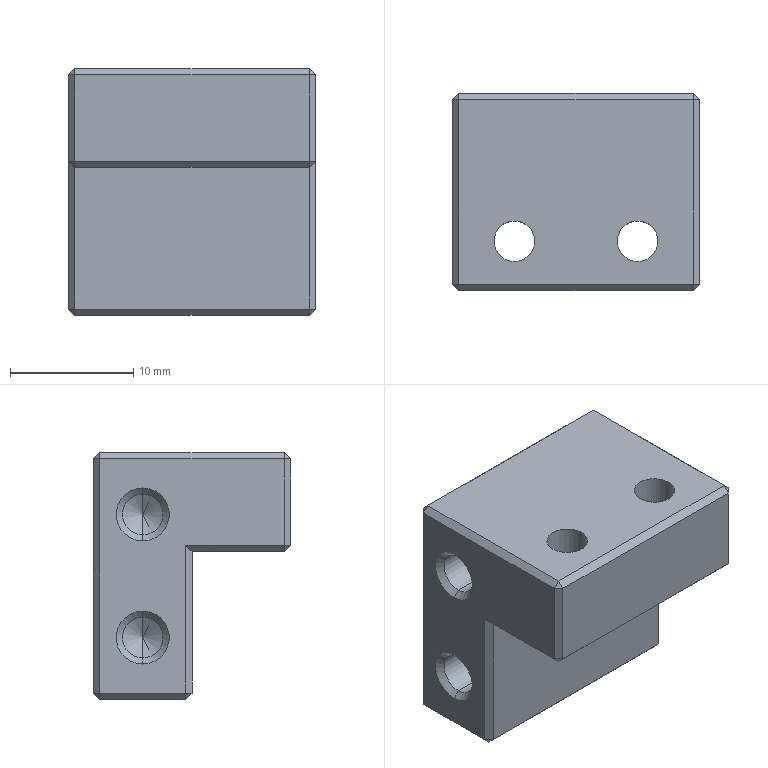Part | SolidWorks | features HoleWzd 2, Chamfer 1, Extrusion 1, ICE 1 | 1 solid | 51 faces | box 20 x 16 x 20 mm | volume 4064 mm3 | plane 35 | cone 8 | cylinder 8 | commonest cylinder face diameters 3.3 x8
STEP:
#1=CARTESIAN_POINT('',(-9.5,4.,-6.65));
#2=VERTEX_POINT('',#1);
#3=CARTESIAN_POINT('',(-9.5,4.,-3.35));
#4=VERTEX_POINT('',#3);
#5=CARTESIAN_POINT('',(-9.5,4.,-5.));
#6=DIRECTION('',(-1.,0.,0.));
#7=DIRECTION('',(0.,0.,-1.));
#8=AXIS2_PLACEMENT_3D('',#5,#6,#7);
#9=CIRCLE('',#8,1.65);
#10=EDGE_CURVE('',#2,#4,#9,.T.);
#11=ORIENTED_EDGE('',*,*,#10,.F.);
#12=CARTESIAN_POINT('',(-10.,4.,-7.15));
#13=VERTEX_POINT('',#12);
#14=CARTESIAN_POINT('',(-9.5,4.,-6.65));
#15=DIRECTION('',(-0.7071,0.,-0.7071));
#16=VECTOR('',#15,1000.);
#17=LINE('',#14,#16);
#18=EDGE_CURVE('',#2,#13,#17,.T.);
#19=ORIENTED_EDGE('',*,*,#18,.T.);
#20=CARTESIAN_POINT('',(-10.,4.,-2.85));
#21=VERTEX_POINT('',#20);
#22=CARTESIAN_POINT('',(-10.,4.,-5.));
#23=DIRECTION('',(1.,0.,0.));
#24=DIRECTION('',(0.,0.,-1.));
#25=AXIS2_PLACEMENT_3D('',#22,#23,#24);
#26=CIRCLE('',#25,2.15);
#27=EDGE_CURVE('',#21,#13,#26,.T.);
#28=ORIENTED_EDGE('',*,*,#27,.F.);
#29=CARTESIAN_POINT('',(-9.5,4.,-3.35));
#30=DIRECTION('',(-0.7071,0.,0.7071));
#31=VECTOR('',#30,1000.);
#32=LINE('',#29,#31);
#33=EDGE_CURVE('',#4,#21,#32,.T.);
#34=ORIENTED_EDGE('',*,*,#33,.F.);
#35=EDGE_LOOP('',(#11,#19,#28,#34));
#36=FACE_OUTER_BOUND('',#35,.T.);
#37=CARTESIAN_POINT('',(-9.5,4.,-5.));
#38=DIRECTION('',(-1.,0.,0.));
#39=DIRECTION('',(0.,0.,1.));
#40=AXIS2_PLACEMENT_3D('',#37,#38,#39);
#41=CONICAL_SURFACE('',#40,1.65,0.7854);
#42=ADVANCED_FACE('',(#36),#41,.F.);
#43=CARTESIAN_POINT('',(-9.5,4.,3.35));
#44=VERTEX_POINT('',#43);
#45=CARTESIAN_POINT('',(-9.5,4.,6.65));
#46=VERTEX_POINT('',#45);
#47=CARTESIAN_POINT('',(-9.5,4.,5.));
#48=DIRECTION('',(-1.,0.,0.));
#49=DIRECTION('',(0.,0.,-1.));
#50=AXIS2_PLACEMENT_3D('',#47,#48,#49);
#51=CIRCLE('',#50,1.65);
#52=EDGE_CURVE('',#44,#46,#51,.T.);
#53=ORIENTED_EDGE('',*,*,#52,.F.);
#54=CARTESIAN_POINT('',(-10.,4.,2.85));
#55=VERTEX_POINT('',#54);
#56=CARTESIAN_POINT('',(-9.5,4.,3.35));
#57=DIRECTION('',(-0.7071,0.,-0.7071));
#58=VECTOR('',#57,1000.);
#59=LINE('',#56,#58);
#60=EDGE_CURVE('',#44,#55,#59,.T.);
#61=ORIENTED_EDGE('',*,*,#60,.T.);
#62=CARTESIAN_POINT('',(-10.,4.,7.15));
#63=VERTEX_POINT('',#62);
#64=CARTESIAN_POINT('',(-10.,4.,5.));
#65=DIRECTION('',(1.,0.,0.));
#66=DIRECTION('',(0.,0.,-1.));
#67=AXIS2_PLACEMENT_3D('',#64,#65,#66);
#68=CIRCLE('',#67,2.15);
#69=EDGE_CURVE('',#63,#55,#68,.T.);
#70=ORIENTED_EDGE('',*,*,#69,.F.);
#71=CARTESIAN_POINT('',(-9.5,4.,6.65));
#72=DIRECTION('',(-0.7071,0.,0.7071));
#73=VECTOR('',#72,1000.);
#74=LINE('',#71,#73);
#75=EDGE_CURVE('',#46,#63,#74,.T.);
#76=ORIENTED_EDGE('',*,*,#75,.F.);
#77=EDGE_LOOP('',(#53,#61,#70,#76));
#78=FACE_OUTER_BOUND('',#77,.T.);
#79=CARTESIAN_POINT('',(-9.5,4.,5.));
#80=DIRECTION('',(-1.,0.,0.));
#81=DIRECTION('',(0.,0.,1.));
#82=AXIS2_PLACEMENT_3D('',#79,#80,#81);
#83=CONICAL_SURFACE('',#82,1.65,0.7854);
#84=ADVANCED_FACE('',(#78),#83,.F.);
#85=CARTESIAN_POINT('',(-6.65,-4.,2.));
#86=VERTEX_POINT('',#85);
#87=CARTESIAN_POINT('',(-3.35,-4.,2.));
#88=VERTEX_POINT('',#87);
#89=CARTESIAN_POINT('',(-5.,-4.,2.));
#90=DIRECTION('',(0.,0.,1.));
#91=DIRECTION('',(1.,0.,0.));
#92=AXIS2_PLACEMENT_3D('',#89,#90,#91);
#93=CIRCLE('',#92,1.65);
#94=EDGE_CURVE('',#86,#88,#93,.T.);
#95=ORIENTED_EDGE('',*,*,#94,.F.);
#96=CARTESIAN_POINT('',(-6.65,-4.,10.));
#97=VERTEX_POINT('',#96);
#98=CARTESIAN_POINT('',(-6.65,-4.,10.));
#99=DIRECTION('',(0.,0.,1.));
#100=VECTOR('',#99,1000.);
#101=LINE('',#98,#100);
#102=EDGE_CURVE('',#86,#97,#101,.T.);
#103=ORIENTED_EDGE('',*,*,#102,.T.);
#104=CARTESIAN_POINT('',(-3.35,-4.,10.));
#105=VERTEX_POINT('',#104);
#106=CARTESIAN_POINT('',(-5.,-4.,10.));
#107=DIRECTION('',(0.,0.,1.));
#108=DIRECTION('',(1.,0.,0.));
#109=AXIS2_PLACEMENT_3D('',#106,#107,#108);
#110=CIRCLE('',#109,1.65);
#111=EDGE_CURVE('',#97,#105,#110,.T.);
#112=ORIENTED_EDGE('',*,*,#111,.T.);
#113=CARTESIAN_POINT('',(-3.35,-4.,10.));
#114=DIRECTION('',(0.,0.,1.));
#115=VECTOR('',#114,1000.);
#116=LINE('',#113,#115);
#117=EDGE_CURVE('',#88,#105,#116,.T.);
#118=ORIENTED_EDGE('',*,*,#117,.F.);
#119=EDGE_LOOP('',(#95,#103,#112,#118));
#120=FACE_OUTER_BOUND('',#119,.T.);
#121=CARTESIAN_POINT('',(-5.,-4.,10.));
#122=DIRECTION('',(0.,0.,1.));
#123=DIRECTION('',(1.,0.,0.));
#124=AXIS2_PLACEMENT_3D('',#121,#122,#123);
#125=CYLINDRICAL_SURFACE('',#124,1.65);
#126=ADVANCED_FACE('',(#120),#125,.F.);
#127=CARTESIAN_POINT('',(3.35,-4.,2.));
#128=VERTEX_POINT('',#127);
#129=CARTESIAN_POINT('',(6.65,-4.,2.));
#130=VERTEX_POINT('',#129);
#131=CARTESIAN_POINT('',(5.,-4.,2.));
#132=DIRECTION('',(0.,0.,1.));
#133=DIRECTION('',(1.,0.,0.));
#134=AXIS2_PLACEMENT_3D('',#131,#132,#133);
#135=CIRCLE('',#134,1.65);
#136=EDGE_CURVE('',#128,#130,#135,.T.);
#137=ORIENTED_EDGE('',*,*,#136,.F.);
#138=CARTESIAN_POINT('',(3.35,-4.,10.));
#139=VERTEX_POINT('',#138);
#140=CARTESIAN_POINT('',(3.35,-4.,10.));
#141=DIRECTION('',(0.,0.,1.));
#142=VECTOR('',#141,1000.);
#143=LINE('',#140,#142);
#144=EDGE_CURVE('',#128,#139,#143,.T.);
#145=ORIENTED_EDGE('',*,*,#144,.T.);
#146=CARTESIAN_POINT('',(6.65,-4.,10.));
#147=VERTEX_POINT('',#146);
#148=CARTESIAN_POINT('',(5.,-4.,10.));
#149=DIRECTION('',(0.,0.,1.));
#150=DIRECTION('',(1.,0.,0.));
#151=AXIS2_PLACEMENT_3D('',#148,#149,#150);
#152=CIRCLE('',#151,1.65);
#153=EDGE_CURVE('',#139,#147,#152,.T.);
#154=ORIENTED_EDGE('',*,*,#153,.T.);
#155=CARTESIAN_POINT('',(6.65,-4.,10.));
#156=DIRECTION('',(0.,0.,1.));
#157=VECTOR('',#156,1000.);
#158=LINE('',#155,#157);
#159=EDGE_CURVE('',#130,#147,#158,.T.);
#160=ORIENTED_EDGE('',*,*,#159,.F.);
#161=EDGE_LOOP('',(#137,#145,#154,#160));
#162=FACE_OUTER_BOUND('',#161,.T.);
#163=CARTESIAN_POINT('',(5.,-4.,10.));
#164=DIRECTION('',(0.,0.,1.));
#165=DIRECTION('',(1.,0.,0.));
#166=AXIS2_PLACEMENT_3D('',#163,#164,#165);
#167=CYLINDRICAL_SURFACE('',#166,1.65);
#168=ADVANCED_FACE('',(#162),#167,.F.);
#169=CARTESIAN_POINT('',(4.1,4.,-6.65));
#170=VERTEX_POINT('',#169);
#171=CARTESIAN_POINT('',(4.1,4.,-3.35));
#172=VERTEX_POINT('',#171);
#173=CARTESIAN_POINT('',(4.1,4.,-5.));
#174=DIRECTION('',(-1.,0.,0.));
#175=DIRECTION('',(0.,0.,1.));
#176=AXIS2_PLACEMENT_3D('',#173,#174,#175);
#177=CIRCLE('',#176,1.65);
#178=EDGE_CURVE('',#170,#172,#177,.T.);
#179=ORIENTED_EDGE('',*,*,#178,.F.);
#180=CARTESIAN_POINT('',(-10.,4.,-6.65));
#181=DIRECTION('',(-1.,0.,0.));
#182=VECTOR('',#181,1000.);
#183=LINE('',#180,#182);
#184=EDGE_CURVE('',#170,#2,#183,.T.);
#185=ORIENTED_EDGE('',*,*,#184,.T.);
#186=ORIENTED_EDGE('',*,*,#10,.T.);
#187=CARTESIAN_POINT('',(-10.,4.,-3.35));
#188=DIRECTION('',(-1.,0.,0.));
#189=VECTOR('',#188,1000.);
#190=LINE('',#187,#189);
#191=EDGE_CURVE('',#172,#4,#190,.T.);
#192=ORIENTED_EDGE('',*,*,#191,.F.);
#193=EDGE_LOOP('',(#179,#185,#186,#192));
#194=FACE_OUTER_BOUND('',#193,.T.);
#195=CARTESIAN_POINT('',(-10.,4.,-5.));
#196=DIRECTION('',(-1.,0.,0.));
#197=DIRECTION('',(0.,0.,1.));
#198=AXIS2_PLACEMENT_3D('',#195,#196,#197);
#199=CYLINDRICAL_SURFACE('',#198,1.65);
#200=ADVANCED_FACE('',(#194),#199,.F.);
#201=CARTESIAN_POINT('',(5.091,4.,-5.));
#202=VERTEX_POINT('',#201);
#203=CARTESIAN_POINT('',(4.1,4.,-3.35));
#204=DIRECTION('',(-0.515,0.,0.8572));
#205=VECTOR('',#204,1000.);
#206=LINE('',#203,#205);
#207=EDGE_CURVE('',#202,#172,#206,.T.);
#208=ORIENTED_EDGE('',*,*,#207,.F.);
#209=CARTESIAN_POINT('',(4.1,4.,-6.65));
#210=DIRECTION('',(-0.515,0.,-0.8572));
#211=VECTOR('',#210,1000.);
#212=LINE('',#209,#211);
#213=EDGE_CURVE('',#202,#170,#212,.T.);
#214=ORIENTED_EDGE('',*,*,#213,.T.);
#215=ORIENTED_EDGE('',*,*,#178,.T.);
#216=EDGE_LOOP('',(#208,#214,#215));
#217=FACE_OUTER_BOUND('',#216,.T.);
#218=CARTESIAN_POINT('',(4.1,4.,-5.));
#219=DIRECTION('',(-1.,0.,0.));
#220=DIRECTION('',(0.,0.,1.));
#221=AXIS2_PLACEMENT_3D('',#218,#219,#220);
#222=CONICAL_SURFACE('',#221,1.65,1.03);
#223=ADVANCED_FACE('',(#217),#222,.F.);
#224=CARTESIAN_POINT('',(4.1,4.,3.35));
#225=VERTEX_POINT('',#224);
#226=CARTESIAN_POINT('',(4.1,4.,6.65));
#227=VERTEX_POINT('',#226);
#228=CARTESIAN_POINT('',(4.1,4.,5.));
#229=DIRECTION('',(-1.,0.,0.));
#230=DIRECTION('',(0.,0.,1.));
#231=AXIS2_PLACEMENT_3D('',#228,#229,#230);
#232=CIRCLE('',#231,1.65);
#233=EDGE_CURVE('',#225,#227,#232,.T.);
#234=ORIENTED_EDGE('',*,*,#233,.F.);
#235=CARTESIAN_POINT('',(-10.,4.,3.35));
#236=DIRECTION('',(-1.,0.,0.));
#237=VECTOR('',#236,1000.);
#238=LINE('',#235,#237);
#239=EDGE_CURVE('',#225,#44,#238,.T.);
#240=ORIENTED_EDGE('',*,*,#239,.T.);
#241=ORIENTED_EDGE('',*,*,#52,.T.);
#242=CARTESIAN_POINT('',(-10.,4.,6.65));
#243=DIRECTION('',(-1.,0.,0.));
#244=VECTOR('',#243,1000.);
#245=LINE('',#242,#244);
#246=EDGE_CURVE('',#227,#46,#245,.T.);
#247=ORIENTED_EDGE('',*,*,#246,.F.);
#248=EDGE_LOOP('',(#234,#240,#241,#247));
#249=FACE_OUTER_BOUND('',#248,.T.);
#250=CARTESIAN_POINT('',(-10.,4.,5.));
#251=DIRECTION('',(-1.,0.,0.));
#252=DIRECTION('',(0.,0.,1.));
#253=AXIS2_PLACEMENT_3D('',#250,#251,#252);
#254=CYLINDRICAL_SURFACE('',#253,1.65);
#255=ADVANCED_FACE('',(#249),#254,.F.);
#256=CARTESIAN_POINT('',(5.091,4.,5.));
#257=VERTEX_POINT('',#256);
#258=CARTESIAN_POINT('',(4.1,4.,6.65));
#259=DIRECTION('',(-0.515,0.,0.8572));
#260=VECTOR('',#259,1000.);
#261=LINE('',#258,#260);
#262=EDGE_CURVE('',#257,#227,#261,.T.);
#263=ORIENTED_EDGE('',*,*,#262,.F.);
#264=CARTESIAN_POINT('',(4.1,4.,3.35));
#265=DIRECTION('',(-0.515,0.,-0.8572));
#266=VECTOR('',#265,1000.);
#267=LINE('',#264,#266);
#268=EDGE_CURVE('',#257,#225,#267,.T.);
#269=ORIENTED_EDGE('',*,*,#268,.T.);
#270=ORIENTED_EDGE('',*,*,#233,.T.);
#271=EDGE_LOOP('',(#263,#269,#270));
#272=FACE_OUTER_BOUND('',#271,.T.);
#273=CARTESIAN_POINT('',(4.1,4.,5.));
#274=DIRECTION('',(-1.,0.,0.));
#275=DIRECTION('',(0.,0.,1.));
#276=AXIS2_PLACEMENT_3D('',#273,#274,#275);
#277=CONICAL_SURFACE('',#276,1.65,1.03);
#278=ADVANCED_FACE('',(#272),#277,.F.);
#279=CARTESIAN_POINT('',(10.,-7.5,2.5));
#280=VERTEX_POINT('',#279);
#281=CARTESIAN_POINT('',(10.,0.5,2.5));
#282=VERTEX_POINT('',#281);
#283=CARTESIAN_POINT('',(10.,8.,2.5));
#284=DIRECTION('',(0.,1.,0.));
#285=VECTOR('',#284,1000.);
#286=LINE('',#283,#285);
#287=EDGE_CURVE('',#280,#282,#286,.T.);
#288=ORIENTED_EDGE('',*,*,#287,.T.);
#289=CARTESIAN_POINT('',(10.,0.5,-9.5));
#290=VERTEX_POINT('',#289);
#291=CARTESIAN_POINT('',(10.,0.5,-10.));
#292=DIRECTION('',(0.,0.,-1.));
#293=VECTOR('',#292,1000.);
#294=LINE('',#291,#293);
#295=EDGE_CURVE('',#282,#290,#294,.T.);
#296=ORIENTED_EDGE('',*,*,#295,.T.);
#297=CARTESIAN_POINT('',(10.,7.5,-9.5));
#298=VERTEX_POINT('',#297);
#299=CARTESIAN_POINT('',(10.,8.,-9.5));
#300=DIRECTION('',(0.,1.,0.));
#301=VECTOR('',#300,1000.);
#302=LINE('',#299,#301);
#303=EDGE_CURVE('',#290,#298,#302,.T.);
#304=ORIENTED_EDGE('',*,*,#303,.T.);
#305=CARTESIAN_POINT('',(10.,7.5,9.5));
#306=VERTEX_POINT('',#305);
#307=CARTESIAN_POINT('',(10.,7.5,10.));
#308=DIRECTION('',(0.,0.,1.));
#309=VECTOR('',#308,1000.);
#310=LINE('',#307,#309);
#311=EDGE_CURVE('',#298,#306,#310,.T.);
#312=ORIENTED_EDGE('',*,*,#311,.T.);
#313=CARTESIAN_POINT('',(10.,-7.5,9.5));
#314=VERTEX_POINT('',#313);
#315=CARTESIAN_POINT('',(10.,8.,9.5));
#316=DIRECTION('',(0.,-1.,0.));
#317=VECTOR('',#316,1000.);
#318=LINE('',#315,#317);
#319=EDGE_CURVE('',#306,#314,#318,.T.);
#320=ORIENTED_EDGE('',*,*,#319,.T.);
#321=CARTESIAN_POINT('',(10.,-7.5,2.));
#322=DIRECTION('',(0.,0.,-1.));
#323=VECTOR('',#322,1000.);
#324=LINE('',#321,#323);
#325=EDGE_CURVE('',#314,#280,#324,.T.);
#326=ORIENTED_EDGE('',*,*,#325,.T.);
#327=EDGE_LOOP('',(#288,#296,#304,#312,#320,#326));
#328=FACE_OUTER_BOUND('',#327,.T.);
#329=CARTESIAN_POINT('',(10.,8.,-10.));
#330=DIRECTION('',(-1.,0.,0.));
#331=DIRECTION('',(0.,0.,1.));
#332=AXIS2_PLACEMENT_3D('',#329,#330,#331);
#333=PLANE('',#332);
#334=ADVANCED_FACE('',(#328),#333,.F.);
#335=CARTESIAN_POINT('',(-9.5,7.5,-10.));
#336=VERTEX_POINT('',#335);
#337=CARTESIAN_POINT('',(9.5,7.5,-10.));
#338=VERTEX_POINT('',#337);
#339=CARTESIAN_POINT('',(10.,7.5,-10.));
#340=DIRECTION('',(1.,0.,0.));
#341=VECTOR('',#340,1000.);
#342=LINE('',#339,#341);
#343=EDGE_CURVE('',#336,#338,#342,.T.);
#344=ORIENTED_EDGE('',*,*,#343,.T.);
#345=CARTESIAN_POINT('',(9.5,0.5,-10.));
#346=VERTEX_POINT('',#345);
#347=CARTESIAN_POINT('',(9.5,8.,-10.));
#348=DIRECTION('',(0.,-1.,0.));
#349=VECTOR('',#348,1000.);
#350=LINE('',#347,#349);
#351=EDGE_CURVE('',#338,#346,#350,.T.);
#352=ORIENTED_EDGE('',*,*,#351,.T.);
#353=CARTESIAN_POINT('',(-9.5,0.5,-10.));
#354=VERTEX_POINT('',#353);
#355=CARTESIAN_POINT('',(-10.,0.5,-10.));
#356=DIRECTION('',(-1.,0.,0.));
#357=VECTOR('',#356,1000.);
#358=LINE('',#355,#357);
#359=EDGE_CURVE('',#346,#354,#358,.T.);
#360=ORIENTED_EDGE('',*,*,#359,.T.);
#361=CARTESIAN_POINT('',(-9.5,8.,-10.));
#362=DIRECTION('',(0.,1.,0.));
#363=VECTOR('',#362,1000.);
#364=LINE('',#361,#363);
#365=EDGE_CURVE('',#354,#336,#364,.T.);
#366=ORIENTED_EDGE('',*,*,#365,.T.);
#367=EDGE_LOOP('',(#344,#352,#360,#366));
#368=FACE_OUTER_BOUND('',#367,.T.);
#369=CARTESIAN_POINT('',(-10.,8.,-10.));
#370=DIRECTION('',(0.,0.,1.));
#371=DIRECTION('',(1.,0.,0.));
#372=AXIS2_PLACEMENT_3D('',#369,#370,#371);
#373=PLANE('',#372);
#374=ADVANCED_FACE('',(#368),#373,.F.);
#375=ORIENTED_EDGE('',*,*,#69,.T.);
#376=CARTESIAN_POINT('',(-10.,4.,5.));
#377=DIRECTION('',(1.,0.,0.));
#378=DIRECTION('',(0.,0.,-1.));
#379=AXIS2_PLACEMENT_3D('',#376,#377,#378);
#380=CIRCLE('',#379,2.15);
#381=EDGE_CURVE('',#55,#63,#380,.T.);
#382=ORIENTED_EDGE('',*,*,#381,.T.);
#383=EDGE_LOOP('',(#375,#382));
#384=FACE_BOUND('',#383,.T.);
#385=ORIENTED_EDGE('',*,*,#27,.T.);
#386=CARTESIAN_POINT('',(-10.,4.,-5.));
#387=DIRECTION('',(1.,0.,0.));
#388=DIRECTION('',(0.,0.,-1.));
#389=AXIS2_PLACEMENT_3D('',#386,#387,#388);
#390=CIRCLE('',#389,2.15);
#391=EDGE_CURVE('',#13,#21,#390,.T.);
#392=ORIENTED_EDGE('',*,*,#391,.T.);
#393=EDGE_LOOP('',(#385,#392));
#394=FACE_BOUND('',#393,.T.);
#395=CARTESIAN_POINT('',(-10.,7.5,-9.5));
#396=VERTEX_POINT('',#395);
#397=CARTESIAN_POINT('',(-10.,0.5,-9.5));
#398=VERTEX_POINT('',#397);
#399=CARTESIAN_POINT('',(-10.,8.,-9.5));
#400=DIRECTION('',(0.,-1.,0.));
#401=VECTOR('',#400,1000.);
#402=LINE('',#399,#401);
#403=EDGE_CURVE('',#396,#398,#402,.T.);
#404=ORIENTED_EDGE('',*,*,#403,.T.);
#405=CARTESIAN_POINT('',(-10.,0.5,2.5));
#406=VERTEX_POINT('',#405);
#407=CARTESIAN_POINT('',(-10.,0.5,-10.));
#408=DIRECTION('',(0.,0.,1.));
#409=VECTOR('',#408,1000.);
#410=LINE('',#407,#409);
#411=EDGE_CURVE('',#398,#406,#410,.T.);
#412=ORIENTED_EDGE('',*,*,#411,.T.);
#413=CARTESIAN_POINT('',(-10.,-7.5,2.5));
#414=VERTEX_POINT('',#413);
#415=CARTESIAN_POINT('',(-10.,8.,2.5));
#416=DIRECTION('',(0.,-1.,0.));
#417=VECTOR('',#416,1000.);
#418=LINE('',#415,#417);
#419=EDGE_CURVE('',#406,#414,#418,.T.);
#420=ORIENTED_EDGE('',*,*,#419,.T.);
#421=CARTESIAN_POINT('',(-10.,-7.5,9.5));
#422=VERTEX_POINT('',#421);
#423=CARTESIAN_POINT('',(-10.,-7.5,10.));
#424=DIRECTION('',(0.,0.,1.));
#425=VECTOR('',#424,1000.);
#426=LINE('',#423,#425);
#427=EDGE_CURVE('',#414,#422,#426,.T.);
#428=ORIENTED_EDGE('',*,*,#427,.T.);
#429=CARTESIAN_POINT('',(-10.,7.5,9.5));
#430=VERTEX_POINT('',#429);
#431=CARTESIAN_POINT('',(-10.,8.,9.5));
#432=DIRECTION('',(0.,1.,0.));
#433=VECTOR('',#432,1000.);
#434=LINE('',#431,#433);
#435=EDGE_CURVE('',#422,#430,#434,.T.);
#436=ORIENTED_EDGE('',*,*,#435,.T.);
#437=CARTESIAN_POINT('',(-10.,7.5,-10.));
#438=DIRECTION('',(0.,0.,-1.));
#439=VECTOR('',#438,1000.);
#440=LINE('',#437,#439);
#441=EDGE_CURVE('',#430,#396,#440,.T.);
#442=ORIENTED_EDGE('',*,*,#441,.T.);
#443=EDGE_LOOP('',(#404,#412,#420,#428,#436,#442));
#444=FACE_OUTER_BOUND('',#443,.T.);
#445=CARTESIAN_POINT('',(-10.,8.,-10.));
#446=DIRECTION('',(1.,0.,0.));
#447=DIRECTION('',(0.,0.,-1.));
#448=AXIS2_PLACEMENT_3D('',#445,#446,#447);
#449=PLANE('',#448);
#450=ADVANCED_FACE('',(#384,#394,#444),#449,.F.);
#451=CARTESIAN_POINT('',(9.5,7.5,10.));
#452=VERTEX_POINT('',#451);
#453=CARTESIAN_POINT('',(-9.5,7.5,10.));
#454=VERTEX_POINT('',#453);
#455=CARTESIAN_POINT('',(-10.,7.5,10.));
#456=DIRECTION('',(-1.,0.,0.));
#457=VECTOR('',#456,1000.);
#458=LINE('',#455,#457);
#459=EDGE_CURVE('',#452,#454,#458,.T.);
#460=ORIENTED_EDGE('',*,*,#459,.T.);
#461=CARTESIAN_POINT('',(-9.5,-7.5,10.));
#462=VERTEX_POINT('',#461);
#463=CARTESIAN_POINT('',(-9.5,8.,10.));
#464=DIRECTION('',(0.,-1.,0.));
#465=VECTOR('',#464,1000.);
#466=LINE('',#463,#465);
#467=EDGE_CURVE('',#454,#462,#466,.T.);
#468=ORIENTED_EDGE('',*,*,#467,.T.);
#469=CARTESIAN_POINT('',(9.5,-7.5,10.));
#470=VERTEX_POINT('',#469);
#471=CARTESIAN_POINT('',(10.,-7.5,10.));
#472=DIRECTION('',(1.,0.,0.));
#473=VECTOR('',#472,1000.);
#474=LINE('',#471,#473);
#475=EDGE_CURVE('',#462,#470,#474,.T.);
#476=ORIENTED_EDGE('',*,*,#475,.T.);
#477=CARTESIAN_POINT('',(9.5,8.,10.));
#478=DIRECTION('',(0.,1.,0.));
#479=VECTOR('',#478,1000.);
#480=LINE('',#477,#479);
#481=EDGE_CURVE('',#470,#452,#480,.T.);
#482=ORIENTED_EDGE('',*,*,#481,.T.);
#483=EDGE_LOOP('',(#460,#468,#476,#482));
#484=FACE_OUTER_BOUND('',#483,.T.);
#485=CARTESIAN_POINT('',(-5.,-4.,10.));
#486=DIRECTION('',(0.,0.,1.));
#487=DIRECTION('',(1.,0.,0.));
#488=AXIS2_PLACEMENT_3D('',#485,#486,#487);
#489=CIRCLE('',#488,1.65);
#490=EDGE_CURVE('',#105,#97,#489,.T.);
#491=ORIENTED_EDGE('',*,*,#490,.F.);
#492=ORIENTED_EDGE('',*,*,#111,.F.);
#493=EDGE_LOOP('',(#491,#492));
#494=FACE_BOUND('',#493,.T.);
#495=CARTESIAN_POINT('',(5.,-4.,10.));
#496=DIRECTION('',(0.,0.,1.));
#497=DIRECTION('',(1.,0.,0.));
#498=AXIS2_PLACEMENT_3D('',#495,#496,#497);
#499=CIRCLE('',#498,1.65);
#500=EDGE_CURVE('',#147,#139,#499,.T.);
#501=ORIENTED_EDGE('',*,*,#500,.F.);
#502=ORIENTED_EDGE('',*,*,#153,.F.);
#503=EDGE_LOOP('',(#501,#502));
#504=FACE_BOUND('',#503,.T.);
#505=CARTESIAN_POINT('',(-10.,8.,10.));
#506=DIRECTION('',(0.,0.,-1.));
#507=DIRECTION('',(-1.,0.,0.));
#508=AXIS2_PLACEMENT_3D('',#505,#506,#507);
#509=PLANE('',#508);
#510=ADVANCED_FACE('',(#484,#494,#504),#509,.F.);
#511=CARTESIAN_POINT('',(9.5,8.,-9.5));
#512=VERTEX_POINT('',#511);
#513=CARTESIAN_POINT('',(-9.5,8.,-9.5));
#514=VERTEX_POINT('',#513);
#515=CARTESIAN_POINT('',(-10.,8.,-9.5));
#516=DIRECTION('',(-1.,0.,0.));
#517=VECTOR('',#516,1000.);
#518=LINE('',#515,#517);
#519=EDGE_CURVE('',#512,#514,#518,.T.);
#520=ORIENTED_EDGE('',*,*,#519,.T.);
#521=CARTESIAN_POINT('',(-9.5,8.,9.5));
#522=VERTEX_POINT('',#521);
#523=CARTESIAN_POINT('',(-9.5,8.,10.));
#524=DIRECTION('',(0.,0.,1.));
#525=VECTOR('',#524,1000.);
#526=LINE('',#523,#525);
#527=EDGE_CURVE('',#514,#522,#526,.T.);
#528=ORIENTED_EDGE('',*,*,#527,.T.);
#529=CARTESIAN_POINT('',(9.5,8.,9.5));
#530=VERTEX_POINT('',#529);
#531=CARTESIAN_POINT('',(10.,8.,9.5));
#532=DIRECTION('',(1.,0.,0.));
#533=VECTOR('',#532,1000.);
#534=LINE('',#531,#533);
#535=EDGE_CURVE('',#522,#530,#534,.T.);
#536=ORIENTED_EDGE('',*,*,#535,.T.);
#537=CARTESIAN_POINT('',(9.5,8.,-10.));
#538=DIRECTION('',(0.,0.,-1.));
#539=VECTOR('',#538,1000.);
#540=LINE('',#537,#539);
#541=EDGE_CURVE('',#530,#512,#540,.T.);
#542=ORIENTED_EDGE('',*,*,#541,.T.);
#543=EDGE_LOOP('',(#520,#528,#536,#542));
#544=FACE_OUTER_BOUND('',#543,.T.);
#545=CARTESIAN_POINT('',(0.,8.,0.));
#546=DIRECTION('',(0.,1.,0.));
#547=DIRECTION('',(0.,0.,1.));
#548=AXIS2_PLACEMENT_3D('',#545,#546,#547);
#549=PLANE('',#548);
#550=ADVANCED_FACE('',(#544),#549,.T.);
#551=CARTESIAN_POINT('',(9.5,0.,2.));
#552=VERTEX_POINT('',#551);
#553=CARTESIAN_POINT('',(-9.5,0.,2.));
#554=VERTEX_POINT('',#553);
#555=CARTESIAN_POINT('',(-10.,0.,2.));
#556=DIRECTION('',(-1.,0.,0.));
#557=VECTOR('',#556,1000.);
#558=LINE('',#555,#557);
#559=EDGE_CURVE('',#552,#554,#558,.T.);
#560=ORIENTED_EDGE('',*,*,#559,.T.);
#561=CARTESIAN_POINT('',(-9.5,0.,-9.5));
#562=VERTEX_POINT('',#561);
#563=CARTESIAN_POINT('',(-9.5,0.,0.));
#564=DIRECTION('',(0.,0.,-1.));
#565=VECTOR('',#564,1000.);
#566=LINE('',#563,#565);
#567=EDGE_CURVE('',#554,#562,#566,.T.);
#568=ORIENTED_EDGE('',*,*,#567,.T.);
#569=CARTESIAN_POINT('',(9.5,0.,-9.5));
#570=VERTEX_POINT('',#569);
#571=CARTESIAN_POINT('',(0.,0.,-9.5));
#572=DIRECTION('',(1.,0.,0.));
#573=VECTOR('',#572,1000.);
#574=LINE('',#571,#573);
#575=EDGE_CURVE('',#562,#570,#574,.T.);
#576=ORIENTED_EDGE('',*,*,#575,.T.);
#577=CARTESIAN_POINT('',(9.5,0.,0.));
#578=DIRECTION('',(0.,0.,1.));
#579=VECTOR('',#578,1000.);
#580=LINE('',#577,#579);
#581=EDGE_CURVE('',#570,#552,#580,.T.);
#582=ORIENTED_EDGE('',*,*,#581,.T.);
#583=EDGE_LOOP('',(#560,#568,#576,#582));
#584=FACE_OUTER_BOUND('',#583,.T.);
#585=CARTESIAN_POINT('',(0.,0.,0.));
#586=DIRECTION('',(0.,1.,0.));
#587=DIRECTION('',(0.,0.,1.));
#588=AXIS2_PLACEMENT_3D('',#585,#586,#587);
#589=PLANE('',#588);
#590=ADVANCED_FACE('',(#584),#589,.F.);
#591=ORIENTED_EDGE('',*,*,#268,.F.);
#592=ORIENTED_EDGE('',*,*,#262,.T.);
#593=CARTESIAN_POINT('',(4.1,4.,5.));
#594=DIRECTION('',(-1.,0.,0.));
#595=DIRECTION('',(0.,0.,1.));
#596=AXIS2_PLACEMENT_3D('',#593,#594,#595);
#597=CIRCLE('',#596,1.65);
#598=EDGE_CURVE('',#227,#225,#597,.T.);
#599=ORIENTED_EDGE('',*,*,#598,.T.);
#600=EDGE_LOOP('',(#591,#592,#599));
#601=FACE_OUTER_BOUND('',#600,.T.);
#602=CARTESIAN_POINT('',(4.1,4.,5.));
#603=DIRECTION('',(-1.,0.,0.));
#604=DIRECTION('',(0.,0.,1.));
#605=AXIS2_PLACEMENT_3D('',#602,#603,#604);
#606=CONICAL_SURFACE('',#605,1.65,1.03);
#607=ADVANCED_FACE('',(#601),#606,.F.);
#608=ORIENTED_EDGE('',*,*,#239,.F.);
#609=ORIENTED_EDGE('',*,*,#598,.F.);
#610=ORIENTED_EDGE('',*,*,#246,.T.);
#611=CARTESIAN_POINT('',(-9.5,4.,5.));
#612=DIRECTION('',(-1.,0.,0.));
#613=DIRECTION('',(0.,0.,-1.));
#614=AXIS2_PLACEMENT_3D('',#611,#612,#613);
#615=CIRCLE('',#614,1.65);
#616=EDGE_CURVE('',#46,#44,#615,.T.);
#617=ORIENTED_EDGE('',*,*,#616,.T.);
#618=EDGE_LOOP('',(#608,#609,#610,#617));
#619=FACE_OUTER_BOUND('',#618,.T.);
#620=CARTESIAN_POINT('',(-10.,4.,5.));
#621=DIRECTION('',(-1.,0.,0.));
#622=DIRECTION('',(0.,0.,1.));
#623=AXIS2_PLACEMENT_3D('',#620,#621,#622);
#624=CYLINDRICAL_SURFACE('',#623,1.65);
#625=ADVANCED_FACE('',(#619),#624,.F.);
#626=ORIENTED_EDGE('',*,*,#213,.F.);
#627=ORIENTED_EDGE('',*,*,#207,.T.);
#628=CARTESIAN_POINT('',(4.1,4.,-5.));
#629=DIRECTION('',(-1.,0.,0.));
#630=DIRECTION('',(0.,0.,1.));
#631=AXIS2_PLACEMENT_3D('',#628,#629,#630);
#632=CIRCLE('',#631,1.65);
#633=EDGE_CURVE('',#172,#170,#632,.T.);
#634=ORIENTED_EDGE('',*,*,#633,.T.);
#635=EDGE_LOOP('',(#626,#627,#634));
#636=FACE_OUTER_BOUND('',#635,.T.);
#637=CARTESIAN_POINT('',(4.1,4.,-5.));
#638=DIRECTION('',(-1.,0.,0.));
#639=DIRECTION('',(0.,0.,1.));
#640=AXIS2_PLACEMENT_3D('',#637,#638,#639);
#641=CONICAL_SURFACE('',#640,1.65,1.03);
#642=ADVANCED_FACE('',(#636),#641,.F.);
#643=ORIENTED_EDGE('',*,*,#184,.F.);
#644=ORIENTED_EDGE('',*,*,#633,.F.);
#645=ORIENTED_EDGE('',*,*,#191,.T.);
#646=CARTESIAN_POINT('',(-9.5,4.,-5.));
#647=DIRECTION('',(-1.,0.,0.));
#648=DIRECTION('',(0.,0.,-1.));
#649=AXIS2_PLACEMENT_3D('',#646,#647,#648);
#650=CIRCLE('',#649,1.65);
#651=EDGE_CURVE('',#4,#2,#650,.T.);
#652=ORIENTED_EDGE('',*,*,#651,.T.);
#653=EDGE_LOOP('',(#643,#644,#645,#652));
#654=FACE_OUTER_BOUND('',#653,.T.);
#655=CARTESIAN_POINT('',(-10.,4.,-5.));
#656=DIRECTION('',(-1.,0.,0.));
#657=DIRECTION('',(0.,0.,1.));
#658=AXIS2_PLACEMENT_3D('',#655,#656,#657);
#659=CYLINDRICAL_SURFACE('',#658,1.65);
#660=ADVANCED_FACE('',(#654),#659,.F.);
#661=CARTESIAN_POINT('',(-9.5,-8.,2.5));
#662=VERTEX_POINT('',#661);
#663=CARTESIAN_POINT('',(9.5,-8.,2.5));
#664=VERTEX_POINT('',#663);
#665=CARTESIAN_POINT('',(10.,-8.,2.5));
#666=DIRECTION('',(1.,0.,0.));
#667=VECTOR('',#666,1000.);
#668=LINE('',#665,#667);
#669=EDGE_CURVE('',#662,#664,#668,.T.);
#670=ORIENTED_EDGE('',*,*,#669,.T.);
#671=CARTESIAN_POINT('',(9.5,-8.,9.5));
#672=VERTEX_POINT('',#671);
#673=CARTESIAN_POINT('',(9.5,-8.,10.));
#674=DIRECTION('',(0.,0.,1.));
#675=VECTOR('',#674,1000.);
#676=LINE('',#673,#675);
#677=EDGE_CURVE('',#664,#672,#676,.T.);
#678=ORIENTED_EDGE('',*,*,#677,.T.);
#679=CARTESIAN_POINT('',(-9.5,-8.,9.5));
#680=VERTEX_POINT('',#679);
#681=CARTESIAN_POINT('',(-10.,-8.,9.5));
#682=DIRECTION('',(-1.,0.,0.));
#683=VECTOR('',#682,1000.);
#684=LINE('',#681,#683);
#685=EDGE_CURVE('',#672,#680,#684,.T.);
#686=ORIENTED_EDGE('',*,*,#685,.T.);
#687=CARTESIAN_POINT('',(-9.5,-8.,2.));
#688=DIRECTION('',(0.,0.,-1.));
#689=VECTOR('',#688,1000.);
#690=LINE('',#687,#689);
#691=EDGE_CURVE('',#680,#662,#690,.T.);
#692=ORIENTED_EDGE('',*,*,#691,.T.);
#693=EDGE_LOOP('',(#670,#678,#686,#692));
#694=FACE_OUTER_BOUND('',#693,.T.);
#695=CARTESIAN_POINT('',(-10.,-8.,2.));
#696=DIRECTION('',(0.,-1.,0.));
#697=DIRECTION('',(0.,0.,-1.));
#698=AXIS2_PLACEMENT_3D('',#695,#696,#697);
#699=PLANE('',#698);
#700=ADVANCED_FACE('',(#694),#699,.T.);
#701=CARTESIAN_POINT('',(-5.,-4.,2.));
#702=DIRECTION('',(0.,0.,1.));
#703=DIRECTION('',(1.,0.,0.));
#704=AXIS2_PLACEMENT_3D('',#701,#702,#703);
#705=CIRCLE('',#704,1.65);
#706=EDGE_CURVE('',#88,#86,#705,.T.);
#707=ORIENTED_EDGE('',*,*,#706,.T.);
#708=ORIENTED_EDGE('',*,*,#94,.T.);
#709=EDGE_LOOP('',(#707,#708));
#710=FACE_BOUND('',#709,.T.);
#711=CARTESIAN_POINT('',(5.,-4.,2.));
#712=DIRECTION('',(0.,0.,1.));
#713=DIRECTION('',(1.,0.,0.));
#714=AXIS2_PLACEMENT_3D('',#711,#712,#713);
#715=CIRCLE('',#714,1.65);
#716=EDGE_CURVE('',#130,#128,#715,.T.);
#717=ORIENTED_EDGE('',*,*,#716,.T.);
#718=ORIENTED_EDGE('',*,*,#136,.T.);
#719=EDGE_LOOP('',(#717,#718));
#720=FACE_BOUND('',#719,.T.);
#721=CARTESIAN_POINT('',(9.5,-7.5,2.));
#722=VERTEX_POINT('',#721);
#723=CARTESIAN_POINT('',(-9.5,-7.5,2.));
#724=VERTEX_POINT('',#723);
#725=CARTESIAN_POINT('',(-10.,-7.5,2.));
#726=DIRECTION('',(-1.,0.,0.));
#727=VECTOR('',#726,1000.);
#728=LINE('',#725,#727);
#729=EDGE_CURVE('',#722,#724,#728,.T.);
#730=ORIENTED_EDGE('',*,*,#729,.T.);
#731=CARTESIAN_POINT('',(-9.5,0.,2.));
#732=DIRECTION('',(0.,1.,0.));
#733=VECTOR('',#732,1000.);
#734=LINE('',#731,#733);
#735=EDGE_CURVE('',#724,#554,#734,.T.);
#736=ORIENTED_EDGE('',*,*,#735,.T.);
#737=ORIENTED_EDGE('',*,*,#559,.F.);
#738=CARTESIAN_POINT('',(9.5,0.,2.));
#739=DIRECTION('',(0.,-1.,0.));
#740=VECTOR('',#739,1000.);
#741=LINE('',#738,#740);
#742=EDGE_CURVE('',#552,#722,#741,.T.);
#743=ORIENTED_EDGE('',*,*,#742,.T.);
#744=EDGE_LOOP('',(#730,#736,#737,#743));
#745=FACE_OUTER_BOUND('',#744,.T.);
#746=CARTESIAN_POINT('',(0.,0.,2.));
#747=DIRECTION('',(0.,0.,1.));
#748=DIRECTION('',(1.,0.,0.));
#749=AXIS2_PLACEMENT_3D('',#746,#747,#748);
#750=PLANE('',#749);
#751=ADVANCED_FACE('',(#710,#720,#745),#750,.F.);
#752=ORIENTED_EDGE('',*,*,#144,.F.);
#753=ORIENTED_EDGE('',*,*,#716,.F.);
#754=ORIENTED_EDGE('',*,*,#159,.T.);
#755=ORIENTED_EDGE('',*,*,#500,.T.);
#756=EDGE_LOOP('',(#752,#753,#754,#755));
#757=FACE_OUTER_BOUND('',#756,.T.);
#758=CARTESIAN_POINT('',(5.,-4.,10.));
#759=DIRECTION('',(0.,0.,1.));
#760=DIRECTION('',(1.,0.,0.));
#761=AXIS2_PLACEMENT_3D('',#758,#759,#760);
#762=CYLINDRICAL_SURFACE('',#761,1.65);
#763=ADVANCED_FACE('',(#757),#762,.F.);
#764=ORIENTED_EDGE('',*,*,#102,.F.);
#765=ORIENTED_EDGE('',*,*,#706,.F.);
#766=ORIENTED_EDGE('',*,*,#117,.T.);
#767=ORIENTED_EDGE('',*,*,#490,.T.);
#768=EDGE_LOOP('',(#764,#765,#766,#767));
#769=FACE_OUTER_BOUND('',#768,.T.);
#770=CARTESIAN_POINT('',(-5.,-4.,10.));
#771=DIRECTION('',(0.,0.,1.));
#772=DIRECTION('',(1.,0.,0.));
#773=AXIS2_PLACEMENT_3D('',#770,#771,#772);
#774=CYLINDRICAL_SURFACE('',#773,1.65);
#775=ADVANCED_FACE('',(#769),#774,.F.);
#776=ORIENTED_EDGE('',*,*,#60,.F.);
#777=ORIENTED_EDGE('',*,*,#616,.F.);
#778=ORIENTED_EDGE('',*,*,#75,.T.);
#779=ORIENTED_EDGE('',*,*,#381,.F.);
#780=EDGE_LOOP('',(#776,#777,#778,#779));
#781=FACE_OUTER_BOUND('',#780,.T.);
#782=CARTESIAN_POINT('',(-9.5,4.,5.));
#783=DIRECTION('',(-1.,0.,0.));
#784=DIRECTION('',(0.,0.,1.));
#785=AXIS2_PLACEMENT_3D('',#782,#783,#784);
#786=CONICAL_SURFACE('',#785,1.65,0.7854);
#787=ADVANCED_FACE('',(#781),#786,.F.);
#788=ORIENTED_EDGE('',*,*,#18,.F.);
#789=ORIENTED_EDGE('',*,*,#651,.F.);
#790=ORIENTED_EDGE('',*,*,#33,.T.);
#791=ORIENTED_EDGE('',*,*,#391,.F.);
#792=EDGE_LOOP('',(#788,#789,#790,#791));
#793=FACE_OUTER_BOUND('',#792,.T.);
#794=CARTESIAN_POINT('',(-9.5,4.,-5.));
#795=DIRECTION('',(-1.,0.,0.));
#796=DIRECTION('',(0.,0.,1.));
#797=AXIS2_PLACEMENT_3D('',#794,#795,#796);
#798=CONICAL_SURFACE('',#797,1.65,0.7854);
#799=ADVANCED_FACE('',(#793),#798,.F.);
#800=CARTESIAN_POINT('',(10.,-7.5,2.5));
#801=DIRECTION('',(0.7071,0.,0.7071));
#802=VECTOR('',#801,1000.);
#803=LINE('',#800,#802);
#804=EDGE_CURVE('',#722,#280,#803,.T.);
#805=ORIENTED_EDGE('',*,*,#804,.F.);
#806=ORIENTED_EDGE('',*,*,#742,.F.);
#807=CARTESIAN_POINT('',(5.833,-3.667,-1.667));
#808=DIRECTION('',(-0.5774,-0.5774,-0.5774));
#809=VECTOR('',#808,1000.);
#810=LINE('',#807,#809);
#811=EDGE_CURVE('',#282,#552,#810,.T.);
#812=ORIENTED_EDGE('',*,*,#811,.F.);
#813=ORIENTED_EDGE('',*,*,#287,.F.);
#814=EDGE_LOOP('',(#805,#806,#812,#813));
#815=FACE_OUTER_BOUND('',#814,.T.);
#816=CARTESIAN_POINT('',(10.,8.,2.5));
#817=DIRECTION('',(-0.7071,0.,0.7071));
#818=DIRECTION('',(0.,1.,0.));
#819=AXIS2_PLACEMENT_3D('',#816,#817,#818);
#820=PLANE('',#819);
#821=ADVANCED_FACE('',(#815),#820,.F.);
#822=CARTESIAN_POINT('',(9.5,-7.75,2.25));
#823=DIRECTION('',(0.,-0.7071,0.7071));
#824=VECTOR('',#823,1000.);
#825=LINE('',#822,#824);
#826=EDGE_CURVE('',#722,#664,#825,.T.);
#827=ORIENTED_EDGE('',*,*,#826,.F.);
#828=ORIENTED_EDGE('',*,*,#804,.T.);
#829=CARTESIAN_POINT('',(10.,-7.5,2.5));
#830=DIRECTION('',(0.7071,0.7071,0.));
#831=VECTOR('',#830,1000.);
#832=LINE('',#829,#831);
#833=EDGE_CURVE('',#664,#280,#832,.T.);
#834=ORIENTED_EDGE('',*,*,#833,.F.);
#835=EDGE_LOOP('',(#827,#828,#834));
#836=FACE_OUTER_BOUND('',#835,.T.);
#837=CARTESIAN_POINT('',(10.,-7.5,2.5));
#838=DIRECTION('',(0.5774,-0.5774,-0.5774));
#839=DIRECTION('',(-0.7071,0.,-0.7071));
#840=AXIS2_PLACEMENT_3D('',#837,#838,#839);
#841=PLANE('',#840);
#842=ADVANCED_FACE('',(#836),#841,.T.);
#843=ORIENTED_EDGE('',*,*,#811,.T.);
#844=ORIENTED_EDGE('',*,*,#581,.F.);
#845=CARTESIAN_POINT('',(9.75,0.25,-9.5));
#846=DIRECTION('',(-0.7071,-0.7071,0.));
#847=VECTOR('',#846,1000.);
#848=LINE('',#845,#847);
#849=EDGE_CURVE('',#290,#570,#848,.T.);
#850=ORIENTED_EDGE('',*,*,#849,.F.);
#851=ORIENTED_EDGE('',*,*,#295,.F.);
#852=EDGE_LOOP('',(#843,#844,#850,#851));
#853=FACE_OUTER_BOUND('',#852,.T.);
#854=CARTESIAN_POINT('',(10.,0.5,-10.));
#855=DIRECTION('',(-0.7071,0.7071,0.));
#856=DIRECTION('',(0.,0.,-1.));
#857=AXIS2_PLACEMENT_3D('',#854,#855,#856);
#858=PLANE('',#857);
#859=ADVANCED_FACE('',(#853),#858,.F.);
#860=ORIENTED_EDGE('',*,*,#833,.T.);
#861=ORIENTED_EDGE('',*,*,#325,.F.);
#862=CARTESIAN_POINT('',(9.5,-8.,9.5));
#863=DIRECTION('',(0.7071,0.7071,0.));
#864=VECTOR('',#863,1000.);
#865=LINE('',#862,#864);
#866=EDGE_CURVE('',#672,#314,#865,.T.);
#867=ORIENTED_EDGE('',*,*,#866,.F.);
#868=ORIENTED_EDGE('',*,*,#677,.F.);
#869=EDGE_LOOP('',(#860,#861,#867,#868));
#870=FACE_OUTER_BOUND('',#869,.T.);
#871=CARTESIAN_POINT('',(9.5,-8.,2.));
#872=DIRECTION('',(0.7071,-0.7071,0.));
#873=DIRECTION('',(0.,0.,-1.));
#874=AXIS2_PLACEMENT_3D('',#871,#872,#873);
#875=PLANE('',#874);
#876=ADVANCED_FACE('',(#870),#875,.T.);
#877=ORIENTED_EDGE('',*,*,#826,.T.);
#878=ORIENTED_EDGE('',*,*,#669,.F.);
#879=CARTESIAN_POINT('',(-9.5,-7.75,2.25));
#880=DIRECTION('',(0.,-0.7071,0.7071));
#881=VECTOR('',#880,1000.);
#882=LINE('',#879,#881);
#883=EDGE_CURVE('',#724,#662,#882,.T.);
#884=ORIENTED_EDGE('',*,*,#883,.F.);
#885=ORIENTED_EDGE('',*,*,#729,.F.);
#886=EDGE_LOOP('',(#877,#878,#884,#885));
#887=FACE_OUTER_BOUND('',#886,.T.);
#888=CARTESIAN_POINT('',(-10.,-8.,2.5));
#889=DIRECTION('',(0.,-0.7071,-0.7071));
#890=DIRECTION('',(-1.,0.,0.));
#891=AXIS2_PLACEMENT_3D('',#888,#889,#890);
#892=PLANE('',#891);
#893=ADVANCED_FACE('',(#887),#892,.T.);
#894=CARTESIAN_POINT('',(-12.5,3.,5.));
#895=DIRECTION('',(-0.5774,0.5774,0.5774));
#896=VECTOR('',#895,1000.);
#897=LINE('',#894,#896);
#898=EDGE_CURVE('',#554,#406,#897,.T.);
#899=ORIENTED_EDGE('',*,*,#898,.F.);
#900=ORIENTED_EDGE('',*,*,#735,.F.);
#901=CARTESIAN_POINT('',(-10.,-7.5,2.5));
#902=DIRECTION('',(0.7071,0.,-0.7071));
#903=VECTOR('',#902,1000.);
#904=LINE('',#901,#903);
#905=EDGE_CURVE('',#414,#724,#904,.T.);
#906=ORIENTED_EDGE('',*,*,#905,.F.);
#907=ORIENTED_EDGE('',*,*,#419,.F.);
#908=EDGE_LOOP('',(#899,#900,#906,#907));
#909=FACE_OUTER_BOUND('',#908,.T.);
#910=CARTESIAN_POINT('',(-10.,8.,2.5));
#911=DIRECTION('',(0.7071,0.,0.7071));
#912=DIRECTION('',(0.,-1.,0.));
#913=AXIS2_PLACEMENT_3D('',#910,#911,#912);
#914=PLANE('',#913);
#915=ADVANCED_FACE('',(#909),#914,.F.);
#916=CARTESIAN_POINT('',(9.5,0.5,-10.));
#917=DIRECTION('',(-0.7071,0.,-0.7071));
#918=VECTOR('',#917,1000.);
#919=LINE('',#916,#918);
#920=EDGE_CURVE('',#290,#346,#919,.T.);
#921=ORIENTED_EDGE('',*,*,#920,.F.);
#922=ORIENTED_EDGE('',*,*,#849,.T.);
#923=CARTESIAN_POINT('',(9.5,0.5,-10.));
#924=DIRECTION('',(0.,-0.7071,0.7071));
#925=VECTOR('',#924,1000.);
#926=LINE('',#923,#925);
#927=EDGE_CURVE('',#346,#570,#926,.T.);
#928=ORIENTED_EDGE('',*,*,#927,.F.);
#929=EDGE_LOOP('',(#921,#922,#928));
#930=FACE_OUTER_BOUND('',#929,.T.);
#931=CARTESIAN_POINT('',(9.5,0.5,-10.));
#932=DIRECTION('',(0.5774,-0.5774,-0.5774));
#933=DIRECTION('',(0.,0.7071,-0.7071));
#934=AXIS2_PLACEMENT_3D('',#931,#932,#933);
#935=PLANE('',#934);
#936=ADVANCED_FACE('',(#930),#935,.T.);
#937=CARTESIAN_POINT('',(9.5,-8.,9.5));
#938=DIRECTION('',(0.,0.7071,0.7071));
#939=VECTOR('',#938,1000.);
#940=LINE('',#937,#939);
#941=EDGE_CURVE('',#672,#470,#940,.T.);
#942=ORIENTED_EDGE('',*,*,#941,.F.);
#943=ORIENTED_EDGE('',*,*,#866,.T.);
#944=CARTESIAN_POINT('',(9.75,-7.5,9.75));
#945=DIRECTION('',(0.7071,0.,-0.7071));
#946=VECTOR('',#945,1000.);
#947=LINE('',#944,#946);
#948=EDGE_CURVE('',#470,#314,#947,.T.);
#949=ORIENTED_EDGE('',*,*,#948,.F.);
#950=EDGE_LOOP('',(#942,#943,#949));
#951=FACE_OUTER_BOUND('',#950,.T.);
#952=CARTESIAN_POINT('',(9.5,-8.,9.5));
#953=DIRECTION('',(0.5774,-0.5774,0.5774));
#954=DIRECTION('',(0.7071,0.,-0.7071));
#955=AXIS2_PLACEMENT_3D('',#952,#953,#954);
#956=PLANE('',#955);
#957=ADVANCED_FACE('',(#951),#956,.T.);
#958=ORIENTED_EDGE('',*,*,#905,.T.);
#959=ORIENTED_EDGE('',*,*,#883,.T.);
#960=CARTESIAN_POINT('',(-10.,-7.5,2.5));
#961=DIRECTION('',(0.7071,-0.7071,0.));
#962=VECTOR('',#961,1000.);
#963=LINE('',#960,#962);
#964=EDGE_CURVE('',#414,#662,#963,.T.);
#965=ORIENTED_EDGE('',*,*,#964,.F.);
#966=EDGE_LOOP('',(#958,#959,#965));
#967=FACE_OUTER_BOUND('',#966,.T.);
#968=CARTESIAN_POINT('',(-10.,-7.5,2.5));
#969=DIRECTION('',(-0.5774,-0.5774,-0.5774));
#970=DIRECTION('',(0.,0.7071,-0.7071));
#971=AXIS2_PLACEMENT_3D('',#968,#969,#970);
#972=PLANE('',#971);
#973=ADVANCED_FACE('',(#967),#972,.T.);
#974=ORIENTED_EDGE('',*,*,#898,.T.);
#975=ORIENTED_EDGE('',*,*,#411,.F.);
#976=CARTESIAN_POINT('',(-9.5,0.,-9.5));
#977=DIRECTION('',(-0.7071,0.7071,0.));
#978=VECTOR('',#977,1000.);
#979=LINE('',#976,#978);
#980=EDGE_CURVE('',#562,#398,#979,.T.);
#981=ORIENTED_EDGE('',*,*,#980,.F.);
#982=ORIENTED_EDGE('',*,*,#567,.F.);
#983=EDGE_LOOP('',(#974,#975,#981,#982));
#984=FACE_OUTER_BOUND('',#983,.T.);
#985=CARTESIAN_POINT('',(-10.,0.5,-10.));
#986=DIRECTION('',(0.7071,0.7071,0.));
#987=DIRECTION('',(0.,0.,1.));
#988=AXIS2_PLACEMENT_3D('',#985,#986,#987);
#989=PLANE('',#988);
#990=ADVANCED_FACE('',(#984),#989,.F.);
#991=ORIENTED_EDGE('',*,*,#927,.T.);
#992=ORIENTED_EDGE('',*,*,#575,.F.);
#993=CARTESIAN_POINT('',(-9.5,0.,-9.5));
#994=DIRECTION('',(0.,-0.7071,0.7071));
#995=VECTOR('',#994,1000.);
#996=LINE('',#993,#995);
#997=EDGE_CURVE('',#354,#562,#996,.T.);
#998=ORIENTED_EDGE('',*,*,#997,.F.);
#999=ORIENTED_EDGE('',*,*,#359,.F.);
#1000=EDGE_LOOP('',(#991,#992,#998,#999));
#1001=FACE_OUTER_BOUND('',#1000,.T.);
#1002=CARTESIAN_POINT('',(-10.,0.5,-10.));
#1003=DIRECTION('',(0.,0.7071,0.7071));
#1004=DIRECTION('',(-1.,0.,0.));
#1005=AXIS2_PLACEMENT_3D('',#1002,#1003,#1004);
#1006=PLANE('',#1005);
#1007=ADVANCED_FACE('',(#1001),#1006,.F.);
#1008=ORIENTED_EDGE('',*,*,#920,.T.);
#1009=ORIENTED_EDGE('',*,*,#351,.F.);
#1010=CARTESIAN_POINT('',(10.,7.5,-9.5));
#1011=DIRECTION('',(-0.7071,0.,-0.7071));
#1012=VECTOR('',#1011,1000.);
#1013=LINE('',#1010,#1012);
#1014=EDGE_CURVE('',#298,#338,#1013,.T.);
#1015=ORIENTED_EDGE('',*,*,#1014,.F.);
#1016=ORIENTED_EDGE('',*,*,#303,.F.);
#1017=EDGE_LOOP('',(#1008,#1009,#1015,#1016));
#1018=FACE_OUTER_BOUND('',#1017,.T.);
#1019=CARTESIAN_POINT('',(9.5,8.,-10.));
#1020=DIRECTION('',(-0.7071,0.,0.7071));
#1021=DIRECTION('',(0.,-1.,0.));
#1022=AXIS2_PLACEMENT_3D('',#1019,#1020,#1021);
#1023=PLANE('',#1022);
#1024=ADVANCED_FACE('',(#1018),#1023,.F.);
#1025=CARTESIAN_POINT('',(10.,7.5,9.5));
#1026=DIRECTION('',(-0.7071,0.7071,0.));
#1027=VECTOR('',#1026,1000.);
#1028=LINE('',#1025,#1027);
#1029=EDGE_CURVE('',#306,#530,#1028,.T.);
#1030=ORIENTED_EDGE('',*,*,#1029,.F.);
#1031=ORIENTED_EDGE('',*,*,#311,.F.);
#1032=CARTESIAN_POINT('',(10.,7.5,-9.5));
#1033=DIRECTION('',(0.7071,-0.7071,0.));
#1034=VECTOR('',#1033,1000.);
#1035=LINE('',#1032,#1034);
#1036=EDGE_CURVE('',#512,#298,#1035,.T.);
#1037=ORIENTED_EDGE('',*,*,#1036,.F.);
#1038=ORIENTED_EDGE('',*,*,#541,.F.);
#1039=EDGE_LOOP('',(#1030,#1031,#1037,#1038));
#1040=FACE_OUTER_BOUND('',#1039,.T.);
#1041=CARTESIAN_POINT('',(9.5,8.,0.));
#1042=DIRECTION('',(0.7071,0.7071,0.));
#1043=DIRECTION('',(0.,0.,1.));
#1044=AXIS2_PLACEMENT_3D('',#1041,#1042,#1043);
#1045=PLANE('',#1044);
#1046=ADVANCED_FACE('',(#1040),#1045,.T.);
#1047=ORIENTED_EDGE('',*,*,#948,.T.);
#1048=ORIENTED_EDGE('',*,*,#319,.F.);
#1049=CARTESIAN_POINT('',(10.,7.5,9.5));
#1050=DIRECTION('',(0.7071,0.,-0.7071));
#1051=VECTOR('',#1050,1000.);
#1052=LINE('',#1049,#1051);
#1053=EDGE_CURVE('',#452,#306,#1052,.T.);
#1054=ORIENTED_EDGE('',*,*,#1053,.F.);
#1055=ORIENTED_EDGE('',*,*,#481,.F.);
#1056=EDGE_LOOP('',(#1047,#1048,#1054,#1055));
#1057=FACE_OUTER_BOUND('',#1056,.T.);
#1058=CARTESIAN_POINT('',(10.,8.,9.5));
#1059=DIRECTION('',(-0.7071,0.,-0.7071));
#1060=DIRECTION('',(0.,-1.,0.));
#1061=AXIS2_PLACEMENT_3D('',#1058,#1059,#1060);
#1062=PLANE('',#1061);
#1063=ADVANCED_FACE('',(#1057),#1062,.F.);
#1064=ORIENTED_EDGE('',*,*,#941,.T.);
#1065=ORIENTED_EDGE('',*,*,#475,.F.);
#1066=CARTESIAN_POINT('',(-9.5,-7.5,10.));
#1067=DIRECTION('',(0.,0.7071,0.7071));
#1068=VECTOR('',#1067,1000.);
#1069=LINE('',#1066,#1068);
#1070=EDGE_CURVE('',#680,#462,#1069,.T.);
#1071=ORIENTED_EDGE('',*,*,#1070,.F.);
#1072=ORIENTED_EDGE('',*,*,#685,.F.);
#1073=EDGE_LOOP('',(#1064,#1065,#1071,#1072));
#1074=FACE_OUTER_BOUND('',#1073,.T.);
#1075=CARTESIAN_POINT('',(-10.,-7.5,10.));
#1076=DIRECTION('',(0.,-0.7071,0.7071));
#1077=DIRECTION('',(-1.,0.,0.));
#1078=AXIS2_PLACEMENT_3D('',#1075,#1076,#1077);
#1079=PLANE('',#1078);
#1080=ADVANCED_FACE('',(#1074),#1079,.T.);
#1081=ORIENTED_EDGE('',*,*,#964,.T.);
#1082=ORIENTED_EDGE('',*,*,#691,.F.);
#1083=CARTESIAN_POINT('',(-9.75,-7.75,9.5));
#1084=DIRECTION('',(0.7071,-0.7071,0.));
#1085=VECTOR('',#1084,1000.);
#1086=LINE('',#1083,#1085);
#1087=EDGE_CURVE('',#422,#680,#1086,.T.);
#1088=ORIENTED_EDGE('',*,*,#1087,.F.);
#1089=ORIENTED_EDGE('',*,*,#427,.F.);
#1090=EDGE_LOOP('',(#1081,#1082,#1088,#1089));
#1091=FACE_OUTER_BOUND('',#1090,.T.);
#1092=CARTESIAN_POINT('',(-10.,-7.5,-10.));
#1093=DIRECTION('',(-0.7071,-0.7071,0.));
#1094=DIRECTION('',(0.,0.,-1.));
#1095=AXIS2_PLACEMENT_3D('',#1092,#1093,#1094);
#1096=PLANE('',#1095);
#1097=ADVANCED_FACE('',(#1091),#1096,.T.);
#1098=ORIENTED_EDGE('',*,*,#997,.T.);
#1099=ORIENTED_EDGE('',*,*,#980,.T.);
#1100=CARTESIAN_POINT('',(-9.75,0.5,-9.75));
#1101=DIRECTION('',(-0.7071,0.,0.7071));
#1102=VECTOR('',#1101,1000.);
#1103=LINE('',#1100,#1102);
#1104=EDGE_CURVE('',#354,#398,#1103,.T.);
#1105=ORIENTED_EDGE('',*,*,#1104,.F.);
#1106=EDGE_LOOP('',(#1098,#1099,#1105));
#1107=FACE_OUTER_BOUND('',#1106,.T.);
#1108=CARTESIAN_POINT('',(-9.5,0.,-9.5));
#1109=DIRECTION('',(-0.5774,-0.5774,-0.5774));
#1110=DIRECTION('',(0.,0.7071,-0.7071));
#1111=AXIS2_PLACEMENT_3D('',#1108,#1109,#1110);
#1112=PLANE('',#1111);
#1113=ADVANCED_FACE('',(#1107),#1112,.T.);
#1114=ORIENTED_EDGE('',*,*,#1036,.T.);
#1115=ORIENTED_EDGE('',*,*,#1014,.T.);
#1116=CARTESIAN_POINT('',(9.5,7.75,-9.75));
#1117=DIRECTION('',(0.,-0.7071,-0.7071));
#1118=VECTOR('',#1117,1000.);
#1119=LINE('',#1116,#1118);
#1120=EDGE_CURVE('',#512,#338,#1119,.T.);
#1121=ORIENTED_EDGE('',*,*,#1120,.F.);
#1122=EDGE_LOOP('',(#1114,#1115,#1121));
#1123=FACE_OUTER_BOUND('',#1122,.T.);
#1124=CARTESIAN_POINT('',(10.,7.5,-9.5));
#1125=DIRECTION('',(0.5774,0.5774,-0.5774));
#1126=DIRECTION('',(0.,0.7071,0.7071));
#1127=AXIS2_PLACEMENT_3D('',#1124,#1125,#1126);
#1128=PLANE('',#1127);
#1129=ADVANCED_FACE('',(#1123),#1128,.T.);
#1130=ORIENTED_EDGE('',*,*,#1053,.T.);
#1131=ORIENTED_EDGE('',*,*,#1029,.T.);
#1132=CARTESIAN_POINT('',(9.5,7.75,9.75));
#1133=DIRECTION('',(0.,0.7071,-0.7071));
#1134=VECTOR('',#1133,1000.);
#1135=LINE('',#1132,#1134);
#1136=EDGE_CURVE('',#452,#530,#1135,.T.);
#1137=ORIENTED_EDGE('',*,*,#1136,.F.);
#1138=EDGE_LOOP('',(#1130,#1131,#1137));
#1139=FACE_OUTER_BOUND('',#1138,.T.);
#1140=CARTESIAN_POINT('',(10.,7.5,9.5));
#1141=DIRECTION('',(0.5774,0.5774,0.5774));
#1142=DIRECTION('',(0.,-0.7071,0.7071));
#1143=AXIS2_PLACEMENT_3D('',#1140,#1141,#1142);
#1144=PLANE('',#1143);
#1145=ADVANCED_FACE('',(#1139),#1144,.T.);
#1146=ORIENTED_EDGE('',*,*,#1087,.T.);
#1147=ORIENTED_EDGE('',*,*,#1070,.T.);
#1148=CARTESIAN_POINT('',(-9.5,-7.5,10.));
#1149=DIRECTION('',(0.7071,0.,0.7071));
#1150=VECTOR('',#1149,1000.);
#1151=LINE('',#1148,#1150);
#1152=EDGE_CURVE('',#422,#462,#1151,.T.);
#1153=ORIENTED_EDGE('',*,*,#1152,.F.);
#1154=EDGE_LOOP('',(#1146,#1147,#1153));
#1155=FACE_OUTER_BOUND('',#1154,.T.);
#1156=CARTESIAN_POINT('',(-9.5,-7.5,10.));
#1157=DIRECTION('',(-0.5774,-0.5774,0.5774));
#1158=DIRECTION('',(0.,-0.7071,-0.7071));
#1159=AXIS2_PLACEMENT_3D('',#1156,#1157,#1158);
#1160=PLANE('',#1159);
#1161=ADVANCED_FACE('',(#1155),#1160,.T.);
#1162=ORIENTED_EDGE('',*,*,#1104,.T.);
#1163=ORIENTED_EDGE('',*,*,#403,.F.);
#1164=CARTESIAN_POINT('',(-10.,7.5,-9.5));
#1165=DIRECTION('',(-0.7071,0.,0.7071));
#1166=VECTOR('',#1165,1000.);
#1167=LINE('',#1164,#1166);
#1168=EDGE_CURVE('',#336,#396,#1167,.T.);
#1169=ORIENTED_EDGE('',*,*,#1168,.F.);
#1170=ORIENTED_EDGE('',*,*,#365,.F.);
#1171=EDGE_LOOP('',(#1162,#1163,#1169,#1170));
#1172=FACE_OUTER_BOUND('',#1171,.T.);
#1173=CARTESIAN_POINT('',(-10.,8.,-9.5));
#1174=DIRECTION('',(0.7071,0.,0.7071));
#1175=DIRECTION('',(0.,-1.,0.));
#1176=AXIS2_PLACEMENT_3D('',#1173,#1174,#1175);
#1177=PLANE('',#1176);
#1178=ADVANCED_FACE('',(#1172),#1177,.F.);
#1179=ORIENTED_EDGE('',*,*,#1120,.T.);
#1180=ORIENTED_EDGE('',*,*,#343,.F.);
#1181=CARTESIAN_POINT('',(-9.5,7.75,-9.75));
#1182=DIRECTION('',(0.,-0.7071,-0.7071));
#1183=VECTOR('',#1182,1000.);
#1184=LINE('',#1181,#1183);
#1185=EDGE_CURVE('',#514,#336,#1184,.T.);
#1186=ORIENTED_EDGE('',*,*,#1185,.F.);
#1187=ORIENTED_EDGE('',*,*,#519,.F.);
#1188=EDGE_LOOP('',(#1179,#1180,#1186,#1187));
#1189=FACE_OUTER_BOUND('',#1188,.T.);
#1190=CARTESIAN_POINT('',(0.,8.,-9.5));
#1191=DIRECTION('',(0.,0.7071,-0.7071));
#1192=DIRECTION('',(1.,0.,0.));
#1193=AXIS2_PLACEMENT_3D('',#1190,#1191,#1192);
#1194=PLANE('',#1193);
#1195=ADVANCED_FACE('',(#1189),#1194,.T.);
#1196=ORIENTED_EDGE('',*,*,#1136,.T.);
#1197=ORIENTED_EDGE('',*,*,#535,.F.);
#1198=CARTESIAN_POINT('',(-9.5,8.,9.5));
#1199=DIRECTION('',(0.,0.7071,-0.7071));
#1200=VECTOR('',#1199,1000.);
#1201=LINE('',#1198,#1200);
#1202=EDGE_CURVE('',#454,#522,#1201,.T.);
#1203=ORIENTED_EDGE('',*,*,#1202,.F.);
#1204=ORIENTED_EDGE('',*,*,#459,.F.);
#1205=EDGE_LOOP('',(#1196,#1197,#1203,#1204));
#1206=FACE_OUTER_BOUND('',#1205,.T.);
#1207=CARTESIAN_POINT('',(0.,8.,9.5));
#1208=DIRECTION('',(0.,0.7071,0.7071));
#1209=DIRECTION('',(-1.,0.,0.));
#1210=AXIS2_PLACEMENT_3D('',#1207,#1208,#1209);
#1211=PLANE('',#1210);
#1212=ADVANCED_FACE('',(#1206),#1211,.T.);
#1213=ORIENTED_EDGE('',*,*,#1152,.T.);
#1214=ORIENTED_EDGE('',*,*,#467,.F.);
#1215=CARTESIAN_POINT('',(-9.75,7.5,9.75));
#1216=DIRECTION('',(0.7071,0.,0.7071));
#1217=VECTOR('',#1216,1000.);
#1218=LINE('',#1215,#1217);
#1219=EDGE_CURVE('',#430,#454,#1218,.T.);
#1220=ORIENTED_EDGE('',*,*,#1219,.F.);
#1221=ORIENTED_EDGE('',*,*,#435,.F.);
#1222=EDGE_LOOP('',(#1213,#1214,#1220,#1221));
#1223=FACE_OUTER_BOUND('',#1222,.T.);
#1224=CARTESIAN_POINT('',(-9.5,8.,10.));
#1225=DIRECTION('',(0.7071,0.,-0.7071));
#1226=DIRECTION('',(0.,-1.,0.));
#1227=AXIS2_PLACEMENT_3D('',#1224,#1225,#1226);
#1228=PLANE('',#1227);
#1229=ADVANCED_FACE('',(#1223),#1228,.F.);
#1230=ORIENTED_EDGE('',*,*,#1185,.T.);
#1231=ORIENTED_EDGE('',*,*,#1168,.T.);
#1232=CARTESIAN_POINT('',(-10.,7.5,-9.5));
#1233=DIRECTION('',(-0.7071,-0.7071,0.));
#1234=VECTOR('',#1233,1000.);
#1235=LINE('',#1232,#1234);
#1236=EDGE_CURVE('',#514,#396,#1235,.T.);
#1237=ORIENTED_EDGE('',*,*,#1236,.F.);
#1238=EDGE_LOOP('',(#1230,#1231,#1237));
#1239=FACE_OUTER_BOUND('',#1238,.T.);
#1240=CARTESIAN_POINT('',(-10.,7.5,-9.5));
#1241=DIRECTION('',(-0.5774,0.5774,-0.5774));
#1242=DIRECTION('',(-0.7071,0.,0.7071));
#1243=AXIS2_PLACEMENT_3D('',#1240,#1241,#1242);
#1244=PLANE('',#1243);
#1245=ADVANCED_FACE('',(#1239),#1244,.T.);
#1246=ORIENTED_EDGE('',*,*,#1219,.T.);
#1247=ORIENTED_EDGE('',*,*,#1202,.T.);
#1248=CARTESIAN_POINT('',(-9.5,8.,9.5));
#1249=DIRECTION('',(0.7071,0.7071,0.));
#1250=VECTOR('',#1249,1000.);
#1251=LINE('',#1248,#1250);
#1252=EDGE_CURVE('',#430,#522,#1251,.T.);
#1253=ORIENTED_EDGE('',*,*,#1252,.F.);
#1254=EDGE_LOOP('',(#1246,#1247,#1253));
#1255=FACE_OUTER_BOUND('',#1254,.T.);
#1256=CARTESIAN_POINT('',(-9.5,8.,9.5));
#1257=DIRECTION('',(-0.5774,0.5774,0.5774));
#1258=DIRECTION('',(0.7071,0.,0.7071));
#1259=AXIS2_PLACEMENT_3D('',#1256,#1257,#1258);
#1260=PLANE('',#1259);
#1261=ADVANCED_FACE('',(#1255),#1260,.T.);
#1262=ORIENTED_EDGE('',*,*,#1236,.T.);
#1263=ORIENTED_EDGE('',*,*,#441,.F.);
#1264=ORIENTED_EDGE('',*,*,#1252,.T.);
#1265=ORIENTED_EDGE('',*,*,#527,.F.);
#1266=EDGE_LOOP('',(#1262,#1263,#1264,#1265));
#1267=FACE_OUTER_BOUND('',#1266,.T.);
#1268=CARTESIAN_POINT('',(-9.5,8.,0.));
#1269=DIRECTION('',(-0.7071,0.7071,0.));
#1270=DIRECTION('',(0.,0.,-1.));
#1271=AXIS2_PLACEMENT_3D('',#1268,#1269,#1270);
#1272=PLANE('',#1271);
#1273=ADVANCED_FACE('',(#1267),#1272,.T.);
#1274=CLOSED_SHELL('',(#42,#84,#126,#168,#200,#223,#255,#278,#334,#374,#450,#510,#550,#590,#607,#625,#642,#660,#700,#751,#763,#775,#787,#799,#821,#842,#859,#876,#893,#915,#936,#957,#973,#990,#1007,#1024,#1046,#1063,#1080,#1097,#1113,#1129,#1145,#1161,#1178,#1195,#1212,#1229,#1245,#1261,#1273));
#1275=MANIFOLD_SOLID_BREP('',#1274);
#1276=CARTESIAN_POINT('',(0.,0.,0.));
#1277=DIRECTION('',(0.,0.,1.));
#1278=DIRECTION('',(1.,0.,0.));
#1279=AXIS2_PLACEMENT_3D('',#1276,#1277,#1278);
#1280=(LENGTH_UNIT()NAMED_UNIT(*)SI_UNIT(.MILLI.,.METRE.));
#1281=UNCERTAINTY_MEASURE_WITH_UNIT(LENGTH_MEASURE(0.00001),#1280,'','');
#1282=(NAMED_UNIT(*)PLANE_ANGLE_UNIT()SI_UNIT($,.RADIAN.));
#1283=(NAMED_UNIT(*)SI_UNIT($,.STERADIAN.)SOLID_ANGLE_UNIT());
#1284=(GEOMETRIC_REPRESENTATION_CONTEXT(3)GLOBAL_UNCERTAINTY_ASSIGNED_CONTEXT((#1281))GLOBAL_UNIT_ASSIGNED_CONTEXT((#1280,#1282,#1283))REPRESENTATION_CONTEXT('',''));
#1285=ADVANCED_BREP_SHAPE_REPRESENTATION('',(#1275,#1279),#1284);